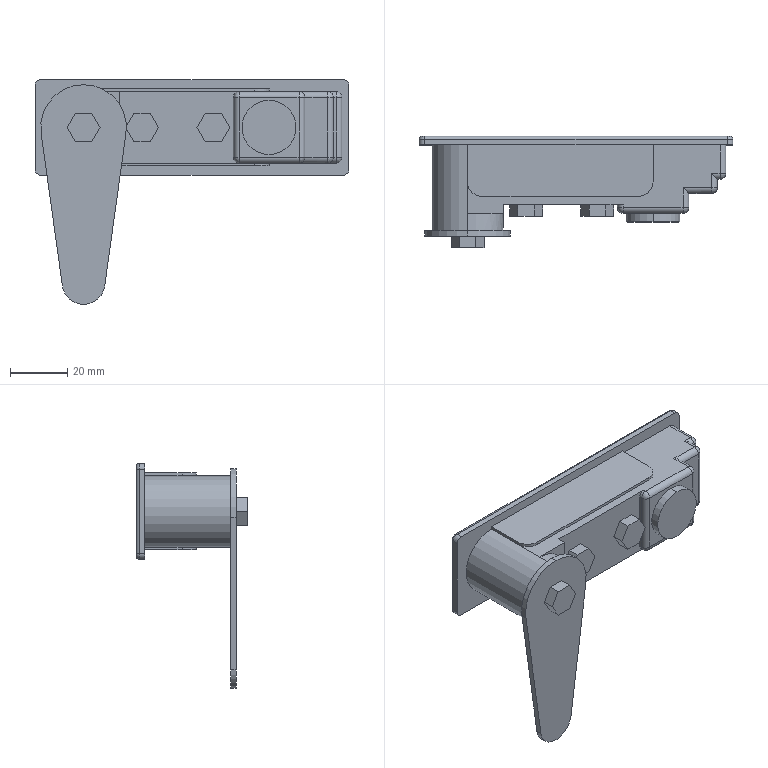Part | SolidWorks | features ICE 11, Fillet 7, BossThin 2, CutThin 2, LPattern 2, CirPattern 1, Emboss 1, Extrusion 1, MirrorPattern 1 | 1 solid | 237 faces | box 110 x 39 x 78.75 mm | volume 72913 mm3 | plane 120 | cylinder 69 | spline 28 | torus 12 | sphere 8 | commonest cylinder face diameters 4 x24 1 x8 1.5 x8 2 x6 10 x5 15 x3